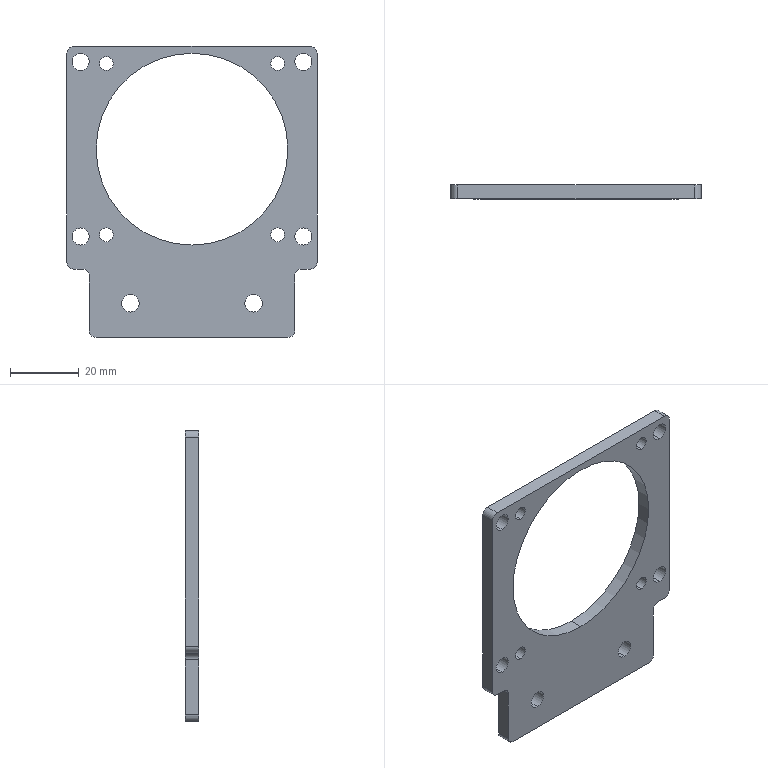Part | STEP file | Drying connection frame | 1 solid | 40 faces | box 73 x 4 x 85 mm | volume 13236 mm3 | cylinder 30 | plane 10 | commonest cylinder face diameters 4 x16 5 x8 5.1 x4 56 x2